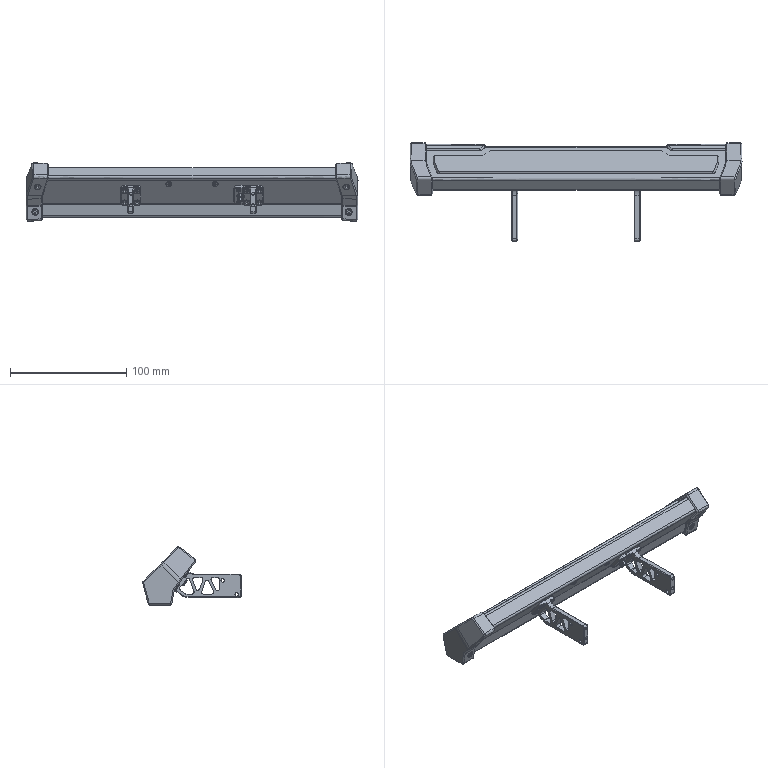Part | SolidWorks | features BaseBody 32, SewRefSurface 2, Thicken 2, DeleteBody 1, ICE 1 | 29 solids | 1636 faces | box 285 x 84.728 x 49.99 mm | volume 138655 mm3 | plane 821 | spline 811 | cylinder 4 | commonest cylinder face diameters 3.2 x4